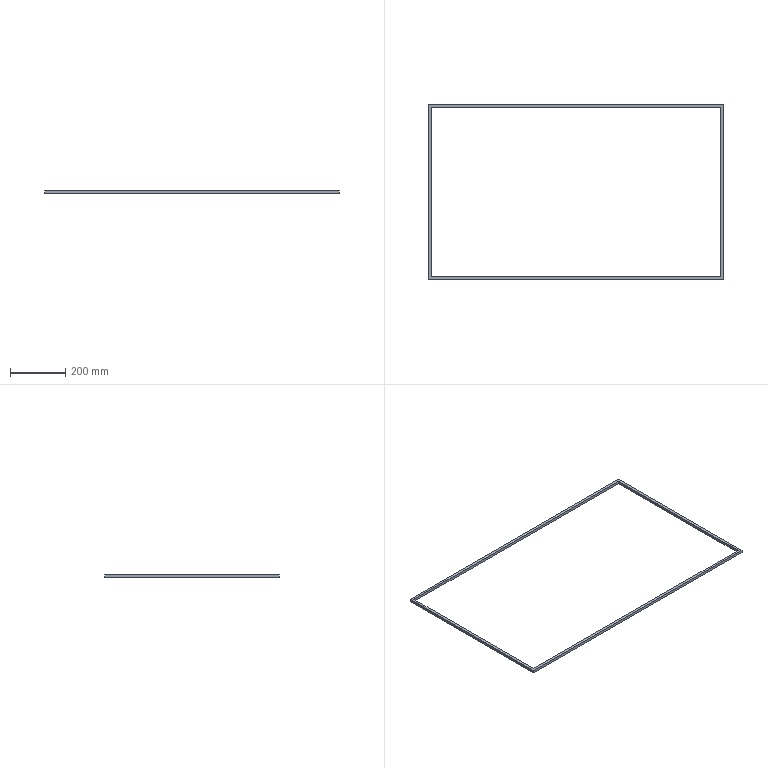Part | SolidWorks | features Extrusion 1 | 1 solid | 10 faces | box 1062 x 630.2 x 10 mm | volume 334440 mm3 | plane 10
STEP:
#1=CARTESIAN_POINT('',(531.,-625.2,10.));
#2=VERTEX_POINT('',#1);
#3=CARTESIAN_POINT('',(531.,5.,10.));
#4=VERTEX_POINT('',#3);
#5=CARTESIAN_POINT('',(531.,-5.,10.));
#6=DIRECTION('',(0.,1.,0.));
#7=VECTOR('',#6,1000.);
#8=LINE('',#5,#7);
#9=EDGE_CURVE('',#2,#4,#8,.T.);
#10=ORIENTED_EDGE('',*,*,#9,.T.);
#11=CARTESIAN_POINT('',(-531.,5.,10.));
#12=VERTEX_POINT('',#11);
#13=CARTESIAN_POINT('',(-531.,5.,10.));
#14=DIRECTION('',(-1.,0.,0.));
#15=VECTOR('',#14,1000.);
#16=LINE('',#13,#15);
#17=EDGE_CURVE('',#4,#12,#16,.T.);
#18=ORIENTED_EDGE('',*,*,#17,.T.);
#19=CARTESIAN_POINT('',(-531.,-625.2,10.));
#20=VERTEX_POINT('',#19);
#21=CARTESIAN_POINT('',(-531.,5.,10.));
#22=DIRECTION('',(0.,-1.,0.));
#23=VECTOR('',#22,1000.);
#24=LINE('',#21,#23);
#25=EDGE_CURVE('',#12,#20,#24,.T.);
#26=ORIENTED_EDGE('',*,*,#25,.T.);
#27=CARTESIAN_POINT('',(-531.,-625.2,10.));
#28=DIRECTION('',(1.,0.,0.));
#29=VECTOR('',#28,1000.);
#30=LINE('',#27,#29);
#31=EDGE_CURVE('',#20,#2,#30,.T.);
#32=ORIENTED_EDGE('',*,*,#31,.T.);
#33=EDGE_LOOP('',(#10,#18,#26,#32));
#34=FACE_OUTER_BOUND('',#33,.T.);
#35=CARTESIAN_POINT('',(521.,-5.,10.));
#36=VERTEX_POINT('',#35);
#37=CARTESIAN_POINT('',(-521.,-5.,10.));
#38=VERTEX_POINT('',#37);
#39=CARTESIAN_POINT('',(-521.,-5.,10.));
#40=DIRECTION('',(-1.,0.,0.));
#41=VECTOR('',#40,1000.);
#42=LINE('',#39,#41);
#43=EDGE_CURVE('',#36,#38,#42,.T.);
#44=ORIENTED_EDGE('',*,*,#43,.F.);
#45=CARTESIAN_POINT('',(521.,-615.2,10.));
#46=VERTEX_POINT('',#45);
#47=CARTESIAN_POINT('',(521.,-5.,10.));
#48=DIRECTION('',(0.,1.,0.));
#49=VECTOR('',#48,1000.);
#50=LINE('',#47,#49);
#51=EDGE_CURVE('',#46,#36,#50,.T.);
#52=ORIENTED_EDGE('',*,*,#51,.F.);
#53=CARTESIAN_POINT('',(-521.,-615.2,10.));
#54=VERTEX_POINT('',#53);
#55=CARTESIAN_POINT('',(-521.,-615.2,10.));
#56=DIRECTION('',(1.,0.,0.));
#57=VECTOR('',#56,1000.);
#58=LINE('',#55,#57);
#59=EDGE_CURVE('',#54,#46,#58,.T.);
#60=ORIENTED_EDGE('',*,*,#59,.F.);
#61=CARTESIAN_POINT('',(-521.,-5.,10.));
#62=DIRECTION('',(0.,-1.,0.));
#63=VECTOR('',#62,1000.);
#64=LINE('',#61,#63);
#65=EDGE_CURVE('',#38,#54,#64,.T.);
#66=ORIENTED_EDGE('',*,*,#65,.F.);
#67=EDGE_LOOP('',(#44,#52,#60,#66));
#68=FACE_BOUND('',#67,.T.);
#69=CARTESIAN_POINT('',(0.,0.,10.));
#70=DIRECTION('',(0.,0.,1.));
#71=DIRECTION('',(1.,0.,0.));
#72=AXIS2_PLACEMENT_3D('',#69,#70,#71);
#73=PLANE('',#72);
#74=ADVANCED_FACE('',(#34,#68),#73,.T.);
#75=CARTESIAN_POINT('',(531.,5.,0.));
#76=VERTEX_POINT('',#75);
#77=CARTESIAN_POINT('',(-531.,5.,0.));
#78=VERTEX_POINT('',#77);
#79=CARTESIAN_POINT('',(-531.,5.,0.));
#80=DIRECTION('',(-1.,0.,0.));
#81=VECTOR('',#80,1000.);
#82=LINE('',#79,#81);
#83=EDGE_CURVE('',#76,#78,#82,.T.);
#84=ORIENTED_EDGE('',*,*,#83,.F.);
#85=CARTESIAN_POINT('',(531.,-625.2,0.));
#86=VERTEX_POINT('',#85);
#87=CARTESIAN_POINT('',(531.,-625.2,0.));
#88=DIRECTION('',(0.,1.,0.));
#89=VECTOR('',#88,1000.);
#90=LINE('',#87,#89);
#91=EDGE_CURVE('',#86,#76,#90,.T.);
#92=ORIENTED_EDGE('',*,*,#91,.F.);
#93=CARTESIAN_POINT('',(-531.,-625.2,0.));
#94=VERTEX_POINT('',#93);
#95=CARTESIAN_POINT('',(-531.,-625.2,0.));
#96=DIRECTION('',(1.,0.,0.));
#97=VECTOR('',#96,1000.);
#98=LINE('',#95,#97);
#99=EDGE_CURVE('',#94,#86,#98,.T.);
#100=ORIENTED_EDGE('',*,*,#99,.F.);
#101=CARTESIAN_POINT('',(-531.,5.,0.));
#102=DIRECTION('',(0.,-1.,0.));
#103=VECTOR('',#102,1000.);
#104=LINE('',#101,#103);
#105=EDGE_CURVE('',#78,#94,#104,.T.);
#106=ORIENTED_EDGE('',*,*,#105,.F.);
#107=EDGE_LOOP('',(#84,#92,#100,#106));
#108=FACE_OUTER_BOUND('',#107,.T.);
#109=CARTESIAN_POINT('',(521.,-615.2,0.));
#110=VERTEX_POINT('',#109);
#111=CARTESIAN_POINT('',(521.,-5.,0.));
#112=VERTEX_POINT('',#111);
#113=CARTESIAN_POINT('',(521.,-5.,0.));
#114=DIRECTION('',(0.,1.,0.));
#115=VECTOR('',#114,1000.);
#116=LINE('',#113,#115);
#117=EDGE_CURVE('',#110,#112,#116,.T.);
#118=ORIENTED_EDGE('',*,*,#117,.T.);
#119=CARTESIAN_POINT('',(-521.,-5.,0.));
#120=VERTEX_POINT('',#119);
#121=CARTESIAN_POINT('',(-521.,-5.,0.));
#122=DIRECTION('',(-1.,0.,0.));
#123=VECTOR('',#122,1000.);
#124=LINE('',#121,#123);
#125=EDGE_CURVE('',#112,#120,#124,.T.);
#126=ORIENTED_EDGE('',*,*,#125,.T.);
#127=CARTESIAN_POINT('',(-521.,-615.2,0.));
#128=VERTEX_POINT('',#127);
#129=CARTESIAN_POINT('',(-521.,-5.,0.));
#130=DIRECTION('',(0.,-1.,0.));
#131=VECTOR('',#130,1000.);
#132=LINE('',#129,#131);
#133=EDGE_CURVE('',#120,#128,#132,.T.);
#134=ORIENTED_EDGE('',*,*,#133,.T.);
#135=CARTESIAN_POINT('',(-521.,-615.2,0.));
#136=DIRECTION('',(1.,0.,0.));
#137=VECTOR('',#136,1000.);
#138=LINE('',#135,#137);
#139=EDGE_CURVE('',#128,#110,#138,.T.);
#140=ORIENTED_EDGE('',*,*,#139,.T.);
#141=EDGE_LOOP('',(#118,#126,#134,#140));
#142=FACE_BOUND('',#141,.T.);
#143=CARTESIAN_POINT('',(0.,0.,0.));
#144=DIRECTION('',(0.,0.,1.));
#145=DIRECTION('',(1.,0.,0.));
#146=AXIS2_PLACEMENT_3D('',#143,#144,#145);
#147=PLANE('',#146);
#148=ADVANCED_FACE('',(#108,#142),#147,.F.);
#149=ORIENTED_EDGE('',*,*,#83,.T.);
#150=CARTESIAN_POINT('',(-531.,5.,10.));
#151=DIRECTION('',(0.,0.,-1.));
#152=VECTOR('',#151,1000.);
#153=LINE('',#150,#152);
#154=EDGE_CURVE('',#12,#78,#153,.T.);
#155=ORIENTED_EDGE('',*,*,#154,.F.);
#156=ORIENTED_EDGE('',*,*,#17,.F.);
#157=CARTESIAN_POINT('',(531.,5.,10.));
#158=DIRECTION('',(0.,0.,-1.));
#159=VECTOR('',#158,1000.);
#160=LINE('',#157,#159);
#161=EDGE_CURVE('',#4,#76,#160,.T.);
#162=ORIENTED_EDGE('',*,*,#161,.T.);
#163=EDGE_LOOP('',(#149,#155,#156,#162));
#164=FACE_OUTER_BOUND('',#163,.T.);
#165=CARTESIAN_POINT('',(-531.,5.,10.));
#166=DIRECTION('',(0.,-1.,0.));
#167=DIRECTION('',(0.,0.,-1.));
#168=AXIS2_PLACEMENT_3D('',#165,#166,#167);
#169=PLANE('',#168);
#170=ADVANCED_FACE('',(#164),#169,.F.);
#171=ORIENTED_EDGE('',*,*,#105,.T.);
#172=CARTESIAN_POINT('',(-531.,-625.2,10.));
#173=DIRECTION('',(0.,0.,-1.));
#174=VECTOR('',#173,1000.);
#175=LINE('',#172,#174);
#176=EDGE_CURVE('',#20,#94,#175,.T.);
#177=ORIENTED_EDGE('',*,*,#176,.F.);
#178=ORIENTED_EDGE('',*,*,#25,.F.);
#179=ORIENTED_EDGE('',*,*,#154,.T.);
#180=EDGE_LOOP('',(#171,#177,#178,#179));
#181=FACE_OUTER_BOUND('',#180,.T.);
#182=CARTESIAN_POINT('',(-531.,5.,10.));
#183=DIRECTION('',(1.,0.,0.));
#184=DIRECTION('',(0.,0.,-1.));
#185=AXIS2_PLACEMENT_3D('',#182,#183,#184);
#186=PLANE('',#185);
#187=ADVANCED_FACE('',(#181),#186,.F.);
#188=ORIENTED_EDGE('',*,*,#99,.T.);
#189=CARTESIAN_POINT('',(531.,-625.2,10.));
#190=DIRECTION('',(0.,0.,-1.));
#191=VECTOR('',#190,1000.);
#192=LINE('',#189,#191);
#193=EDGE_CURVE('',#2,#86,#192,.T.);
#194=ORIENTED_EDGE('',*,*,#193,.F.);
#195=ORIENTED_EDGE('',*,*,#31,.F.);
#196=ORIENTED_EDGE('',*,*,#176,.T.);
#197=EDGE_LOOP('',(#188,#194,#195,#196));
#198=FACE_OUTER_BOUND('',#197,.T.);
#199=CARTESIAN_POINT('',(-531.,-625.2,10.));
#200=DIRECTION('',(0.,1.,0.));
#201=DIRECTION('',(0.,0.,1.));
#202=AXIS2_PLACEMENT_3D('',#199,#200,#201);
#203=PLANE('',#202);
#204=ADVANCED_FACE('',(#198),#203,.F.);
#205=ORIENTED_EDGE('',*,*,#91,.T.);
#206=ORIENTED_EDGE('',*,*,#161,.F.);
#207=ORIENTED_EDGE('',*,*,#9,.F.);
#208=ORIENTED_EDGE('',*,*,#193,.T.);
#209=EDGE_LOOP('',(#205,#206,#207,#208));
#210=FACE_OUTER_BOUND('',#209,.T.);
#211=CARTESIAN_POINT('',(531.,-625.2,10.));
#212=DIRECTION('',(-1.,0.,0.));
#213=DIRECTION('',(0.,0.,1.));
#214=AXIS2_PLACEMENT_3D('',#211,#212,#213);
#215=PLANE('',#214);
#216=ADVANCED_FACE('',(#210),#215,.F.);
#217=ORIENTED_EDGE('',*,*,#117,.F.);
#218=CARTESIAN_POINT('',(521.,-615.2,10.));
#219=DIRECTION('',(0.,0.,-1.));
#220=VECTOR('',#219,1000.);
#221=LINE('',#218,#220);
#222=EDGE_CURVE('',#46,#110,#221,.T.);
#223=ORIENTED_EDGE('',*,*,#222,.F.);
#224=ORIENTED_EDGE('',*,*,#51,.T.);
#225=CARTESIAN_POINT('',(521.,-5.,10.));
#226=DIRECTION('',(0.,0.,-1.));
#227=VECTOR('',#226,1000.);
#228=LINE('',#225,#227);
#229=EDGE_CURVE('',#36,#112,#228,.T.);
#230=ORIENTED_EDGE('',*,*,#229,.T.);
#231=EDGE_LOOP('',(#217,#223,#224,#230));
#232=FACE_OUTER_BOUND('',#231,.T.);
#233=CARTESIAN_POINT('',(521.,-5.,10.));
#234=DIRECTION('',(-1.,0.,0.));
#235=DIRECTION('',(0.,0.,1.));
#236=AXIS2_PLACEMENT_3D('',#233,#234,#235);
#237=PLANE('',#236);
#238=ADVANCED_FACE('',(#232),#237,.T.);
#239=ORIENTED_EDGE('',*,*,#125,.F.);
#240=ORIENTED_EDGE('',*,*,#229,.F.);
#241=ORIENTED_EDGE('',*,*,#43,.T.);
#242=CARTESIAN_POINT('',(-521.,-5.,10.));
#243=DIRECTION('',(0.,0.,-1.));
#244=VECTOR('',#243,1000.);
#245=LINE('',#242,#244);
#246=EDGE_CURVE('',#38,#120,#245,.T.);
#247=ORIENTED_EDGE('',*,*,#246,.T.);
#248=EDGE_LOOP('',(#239,#240,#241,#247));
#249=FACE_OUTER_BOUND('',#248,.T.);
#250=CARTESIAN_POINT('',(-521.,-5.,10.));
#251=DIRECTION('',(0.,-1.,0.));
#252=DIRECTION('',(1.,0.,0.));
#253=AXIS2_PLACEMENT_3D('',#250,#251,#252);
#254=PLANE('',#253);
#255=ADVANCED_FACE('',(#249),#254,.T.);
#256=ORIENTED_EDGE('',*,*,#133,.F.);
#257=ORIENTED_EDGE('',*,*,#246,.F.);
#258=ORIENTED_EDGE('',*,*,#65,.T.);
#259=CARTESIAN_POINT('',(-521.,-615.2,10.));
#260=DIRECTION('',(0.,0.,-1.));
#261=VECTOR('',#260,1000.);
#262=LINE('',#259,#261);
#263=EDGE_CURVE('',#54,#128,#262,.T.);
#264=ORIENTED_EDGE('',*,*,#263,.T.);
#265=EDGE_LOOP('',(#256,#257,#258,#264));
#266=FACE_OUTER_BOUND('',#265,.T.);
#267=CARTESIAN_POINT('',(-521.,-5.,10.));
#268=DIRECTION('',(1.,0.,0.));
#269=DIRECTION('',(0.,0.,-1.));
#270=AXIS2_PLACEMENT_3D('',#267,#268,#269);
#271=PLANE('',#270);
#272=ADVANCED_FACE('',(#266),#271,.T.);
#273=ORIENTED_EDGE('',*,*,#139,.F.);
#274=ORIENTED_EDGE('',*,*,#263,.F.);
#275=ORIENTED_EDGE('',*,*,#59,.T.);
#276=ORIENTED_EDGE('',*,*,#222,.T.);
#277=EDGE_LOOP('',(#273,#274,#275,#276));
#278=FACE_OUTER_BOUND('',#277,.T.);
#279=CARTESIAN_POINT('',(-521.,-615.2,10.));
#280=DIRECTION('',(0.,1.,0.));
#281=DIRECTION('',(0.,0.,1.));
#282=AXIS2_PLACEMENT_3D('',#279,#280,#281);
#283=PLANE('',#282);
#284=ADVANCED_FACE('',(#278),#283,.T.);
#285=CLOSED_SHELL('',(#74,#148,#170,#187,#204,#216,#238,#255,#272,#284));
#286=MANIFOLD_SOLID_BREP('',#285);
#287=CARTESIAN_POINT('',(0.,0.,0.));
#288=DIRECTION('',(0.,0.,1.));
#289=DIRECTION('',(1.,0.,0.));
#290=AXIS2_PLACEMENT_3D('',#287,#288,#289);
#291=(LENGTH_UNIT()NAMED_UNIT(*)SI_UNIT(.MILLI.,.METRE.));
#292=UNCERTAINTY_MEASURE_WITH_UNIT(LENGTH_MEASURE(0.00001),#291,'','');
#293=(NAMED_UNIT(*)PLANE_ANGLE_UNIT()SI_UNIT($,.RADIAN.));
#294=(NAMED_UNIT(*)SI_UNIT($,.STERADIAN.)SOLID_ANGLE_UNIT());
#295=(GEOMETRIC_REPRESENTATION_CONTEXT(3)GLOBAL_UNCERTAINTY_ASSIGNED_CONTEXT((#292))GLOBAL_UNIT_ASSIGNED_CONTEXT((#291,#293,#294))REPRESENTATION_CONTEXT('',''));
#296=ADVANCED_BREP_SHAPE_REPRESENTATION('',(#286,#290),#295);